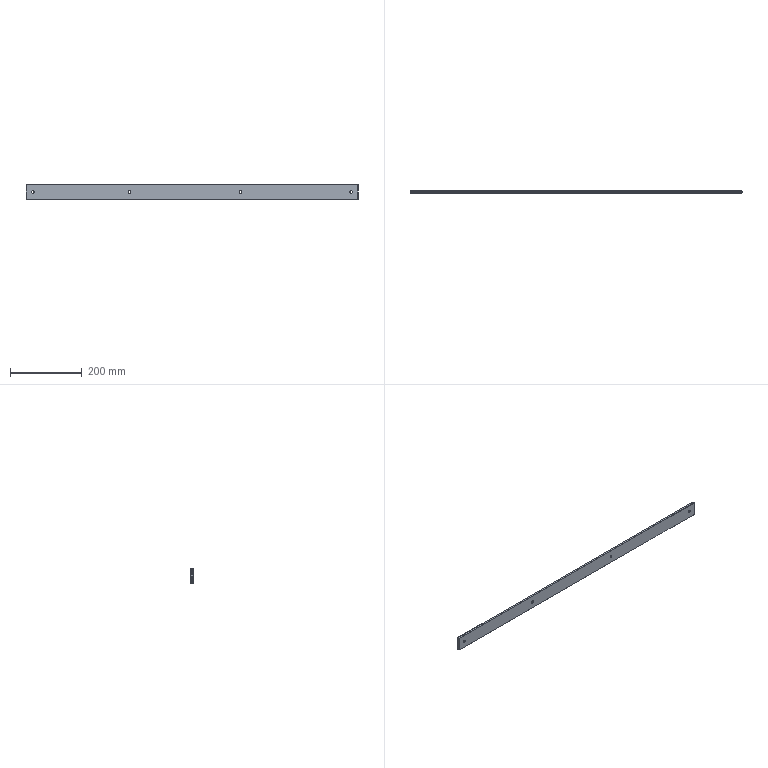Part | NX | 1 solid | 26 faces | box 928 x 6 x 40 mm | volume 221621 mm3 | plane 18 | cylinder 8 | commonest cylinder face diameters 7 x8
STEP:
#1=CARTESIAN_POINT('',(927.7,0.,-19.7));
#2=VERTEX_POINT('',#1);
#3=CARTESIAN_POINT('',(927.7,0.,19.7));
#4=VERTEX_POINT('',#3);
#5=CARTESIAN_POINT('',(927.7,0.,0.));
#6=DIRECTION('',(0.,0.,1.));
#7=VECTOR('',#6,1000.);
#8=LINE('',#5,#7);
#9=EDGE_CURVE('',#2,#4,#8,.T.);
#10=ORIENTED_EDGE('',*,*,#9,.T.);
#11=CARTESIAN_POINT('',(0.3,0.,19.7));
#12=VERTEX_POINT('',#11);
#13=CARTESIAN_POINT('',(464.,0.,19.7));
#14=DIRECTION('',(-1.,0.,0.));
#15=VECTOR('',#14,1000.);
#16=LINE('',#13,#15);
#17=EDGE_CURVE('',#4,#12,#16,.T.);
#18=ORIENTED_EDGE('',*,*,#17,.T.);
#19=CARTESIAN_POINT('',(0.3,0.,-19.7));
#20=VERTEX_POINT('',#19);
#21=CARTESIAN_POINT('',(0.3,0.,0.));
#22=DIRECTION('',(0.,0.,-1.));
#23=VECTOR('',#22,1000.);
#24=LINE('',#21,#23);
#25=EDGE_CURVE('',#12,#20,#24,.T.);
#26=ORIENTED_EDGE('',*,*,#25,.T.);
#27=CARTESIAN_POINT('',(464.,0.,-19.7));
#28=DIRECTION('',(1.,0.,0.));
#29=VECTOR('',#28,1000.);
#30=LINE('',#27,#29);
#31=EDGE_CURVE('',#20,#2,#30,.T.);
#32=ORIENTED_EDGE('',*,*,#31,.T.);
#33=EDGE_LOOP('',(#10,#18,#26,#32));
#34=FACE_BOUND('',#33,.T.);
#35=CARTESIAN_POINT('',(912.5,0.,0.));
#36=VERTEX_POINT('',#35);
#37=CARTESIAN_POINT('',(905.5,0.,0.));
#38=VERTEX_POINT('',#37);
#39=CARTESIAN_POINT('',(909.,0.,0.));
#40=DIRECTION('',(0.,-1.,0.));
#41=DIRECTION('',(-1.,0.,0.));
#42=AXIS2_PLACEMENT_3D('',#39,#40,#41);
#43=CIRCLE('',#42,3.5);
#44=EDGE_CURVE('',#36,#38,#43,.T.);
#45=ORIENTED_EDGE('',*,*,#44,.F.);
#46=CARTESIAN_POINT('',(909.,0.,0.));
#47=DIRECTION('',(0.,-1.,0.));
#48=DIRECTION('',(-1.,0.,0.));
#49=AXIS2_PLACEMENT_3D('',#46,#47,#48);
#50=CIRCLE('',#49,3.5);
#51=EDGE_CURVE('',#38,#36,#50,.T.);
#52=ORIENTED_EDGE('',*,*,#51,.F.);
#53=EDGE_LOOP('',(#45,#52));
#54=FACE_BOUND('',#53,.T.);
#55=CARTESIAN_POINT('',(595.5,0.,0.));
#56=VERTEX_POINT('',#55);
#57=CARTESIAN_POINT('',(602.5,0.,0.));
#58=VERTEX_POINT('',#57);
#59=CARTESIAN_POINT('',(599.,0.,0.));
#60=DIRECTION('',(0.,-1.,0.));
#61=DIRECTION('',(-1.,0.,0.));
#62=AXIS2_PLACEMENT_3D('',#59,#60,#61);
#63=CIRCLE('',#62,3.5);
#64=EDGE_CURVE('',#56,#58,#63,.T.);
#65=ORIENTED_EDGE('',*,*,#64,.F.);
#66=CARTESIAN_POINT('',(599.,0.,0.));
#67=DIRECTION('',(0.,-1.,0.));
#68=DIRECTION('',(-1.,0.,0.));
#69=AXIS2_PLACEMENT_3D('',#66,#67,#68);
#70=CIRCLE('',#69,3.5);
#71=EDGE_CURVE('',#58,#56,#70,.T.);
#72=ORIENTED_EDGE('',*,*,#71,.F.);
#73=EDGE_LOOP('',(#65,#72));
#74=FACE_BOUND('',#73,.T.);
#75=CARTESIAN_POINT('',(285.5,0.,0.));
#76=VERTEX_POINT('',#75);
#77=CARTESIAN_POINT('',(292.5,0.,0.));
#78=VERTEX_POINT('',#77);
#79=CARTESIAN_POINT('',(289.,0.,0.));
#80=DIRECTION('',(0.,-1.,0.));
#81=DIRECTION('',(-1.,0.,0.));
#82=AXIS2_PLACEMENT_3D('',#79,#80,#81);
#83=CIRCLE('',#82,3.5);
#84=EDGE_CURVE('',#76,#78,#83,.T.);
#85=ORIENTED_EDGE('',*,*,#84,.F.);
#86=CARTESIAN_POINT('',(289.,0.,0.));
#87=DIRECTION('',(0.,-1.,0.));
#88=DIRECTION('',(-1.,0.,0.));
#89=AXIS2_PLACEMENT_3D('',#86,#87,#88);
#90=CIRCLE('',#89,3.5);
#91=EDGE_CURVE('',#78,#76,#90,.T.);
#92=ORIENTED_EDGE('',*,*,#91,.F.);
#93=EDGE_LOOP('',(#85,#92));
#94=FACE_BOUND('',#93,.T.);
#95=CARTESIAN_POINT('',(22.5,0.,0.));
#96=VERTEX_POINT('',#95);
#97=CARTESIAN_POINT('',(15.5,0.,0.));
#98=VERTEX_POINT('',#97);
#99=CARTESIAN_POINT('',(19.,0.,0.));
#100=DIRECTION('',(0.,-1.,0.));
#101=DIRECTION('',(-1.,0.,0.));
#102=AXIS2_PLACEMENT_3D('',#99,#100,#101);
#103=CIRCLE('',#102,3.5);
#104=EDGE_CURVE('',#96,#98,#103,.T.);
#105=ORIENTED_EDGE('',*,*,#104,.F.);
#106=CARTESIAN_POINT('',(19.,0.,0.));
#107=DIRECTION('',(0.,-1.,0.));
#108=DIRECTION('',(-1.,0.,0.));
#109=AXIS2_PLACEMENT_3D('',#106,#107,#108);
#110=CIRCLE('',#109,3.5);
#111=EDGE_CURVE('',#98,#96,#110,.T.);
#112=ORIENTED_EDGE('',*,*,#111,.F.);
#113=EDGE_LOOP('',(#105,#112));
#114=FACE_BOUND('',#113,.T.);
#115=CARTESIAN_POINT('',(0.,0.,0.));
#116=DIRECTION('',(0.,1.,0.));
#117=DIRECTION('',(1.,0.,0.));
#118=AXIS2_PLACEMENT_3D('',#115,#116,#117);
#119=PLANE('',#118);
#120=ADVANCED_FACE('',(#34,#54,#74,#94,#114),#119,.F.);
#121=CARTESIAN_POINT('',(0.,5.7,19.7));
#122=VERTEX_POINT('',#121);
#123=CARTESIAN_POINT('',(0.,0.3,19.7));
#124=VERTEX_POINT('',#123);
#125=CARTESIAN_POINT('',(0.,3.,19.7));
#126=DIRECTION('',(0.,-1.,0.));
#127=VECTOR('',#126,1000.);
#128=LINE('',#125,#127);
#129=EDGE_CURVE('',#122,#124,#128,.T.);
#130=ORIENTED_EDGE('',*,*,#129,.F.);
#131=CARTESIAN_POINT('',(0.,5.7,-19.7));
#132=VERTEX_POINT('',#131);
#133=CARTESIAN_POINT('',(0.,5.7,0.));
#134=DIRECTION('',(0.,0.,-1.));
#135=VECTOR('',#134,1000.);
#136=LINE('',#133,#135);
#137=EDGE_CURVE('',#122,#132,#136,.T.);
#138=ORIENTED_EDGE('',*,*,#137,.T.);
#139=CARTESIAN_POINT('',(0.,0.3,-19.7));
#140=VERTEX_POINT('',#139);
#141=CARTESIAN_POINT('',(0.,3.,-19.7));
#142=DIRECTION('',(0.,-1.,0.));
#143=VECTOR('',#142,1000.);
#144=LINE('',#141,#143);
#145=EDGE_CURVE('',#132,#140,#144,.T.);
#146=ORIENTED_EDGE('',*,*,#145,.T.);
#147=CARTESIAN_POINT('',(0.,0.3,0.));
#148=DIRECTION('',(0.,0.,-1.));
#149=VECTOR('',#148,1000.);
#150=LINE('',#147,#149);
#151=EDGE_CURVE('',#124,#140,#150,.T.);
#152=ORIENTED_EDGE('',*,*,#151,.F.);
#153=EDGE_LOOP('',(#130,#138,#146,#152));
#154=FACE_BOUND('',#153,.T.);
#155=CARTESIAN_POINT('',(0.,0.,-20.));
#156=DIRECTION('',(-1.,0.,0.));
#157=DIRECTION('',(0.,0.,1.));
#158=AXIS2_PLACEMENT_3D('',#155,#156,#157);
#159=PLANE('',#158);
#160=ADVANCED_FACE('',(#154),#159,.T.);
#161=CARTESIAN_POINT('',(927.7,5.7,-20.));
#162=VERTEX_POINT('',#161);
#163=CARTESIAN_POINT('',(927.7,0.3,-20.));
#164=VERTEX_POINT('',#163);
#165=CARTESIAN_POINT('',(927.7,3.,-20.));
#166=DIRECTION('',(0.,-1.,0.));
#167=VECTOR('',#166,1000.);
#168=LINE('',#165,#167);
#169=EDGE_CURVE('',#162,#164,#168,.T.);
#170=ORIENTED_EDGE('',*,*,#169,.T.);
#171=CARTESIAN_POINT('',(0.3,0.3,-20.));
#172=VERTEX_POINT('',#171);
#173=CARTESIAN_POINT('',(464.,0.3,-20.));
#174=DIRECTION('',(1.,0.,0.));
#175=VECTOR('',#174,1000.);
#176=LINE('',#173,#175);
#177=EDGE_CURVE('',#172,#164,#176,.T.);
#178=ORIENTED_EDGE('',*,*,#177,.F.);
#179=CARTESIAN_POINT('',(0.3,5.7,-20.));
#180=VERTEX_POINT('',#179);
#181=CARTESIAN_POINT('',(0.3,3.,-20.));
#182=DIRECTION('',(0.,-1.,0.));
#183=VECTOR('',#182,1000.);
#184=LINE('',#181,#183);
#185=EDGE_CURVE('',#180,#172,#184,.T.);
#186=ORIENTED_EDGE('',*,*,#185,.F.);
#187=CARTESIAN_POINT('',(464.,5.7,-20.));
#188=DIRECTION('',(1.,0.,0.));
#189=VECTOR('',#188,1000.);
#190=LINE('',#187,#189);
#191=EDGE_CURVE('',#180,#162,#190,.T.);
#192=ORIENTED_EDGE('',*,*,#191,.T.);
#193=EDGE_LOOP('',(#170,#178,#186,#192));
#194=FACE_BOUND('',#193,.T.);
#195=CARTESIAN_POINT('',(928.,0.,-20.));
#196=DIRECTION('',(0.,0.,-1.));
#197=DIRECTION('',(0.,-1.,0.));
#198=AXIS2_PLACEMENT_3D('',#195,#196,#197);
#199=PLANE('',#198);
#200=ADVANCED_FACE('',(#194),#199,.T.);
#201=CARTESIAN_POINT('',(928.,5.7,-19.7));
#202=VERTEX_POINT('',#201);
#203=CARTESIAN_POINT('',(928.,5.7,19.7));
#204=VERTEX_POINT('',#203);
#205=CARTESIAN_POINT('',(928.,5.7,0.));
#206=DIRECTION('',(0.,0.,1.));
#207=VECTOR('',#206,1000.);
#208=LINE('',#205,#207);
#209=EDGE_CURVE('',#202,#204,#208,.T.);
#210=ORIENTED_EDGE('',*,*,#209,.T.);
#211=CARTESIAN_POINT('',(928.,0.3,19.7));
#212=VERTEX_POINT('',#211);
#213=CARTESIAN_POINT('',(928.,3.,19.7));
#214=DIRECTION('',(0.,-1.,0.));
#215=VECTOR('',#214,1000.);
#216=LINE('',#213,#215);
#217=EDGE_CURVE('',#204,#212,#216,.T.);
#218=ORIENTED_EDGE('',*,*,#217,.T.);
#219=CARTESIAN_POINT('',(928.,0.3,-19.7));
#220=VERTEX_POINT('',#219);
#221=CARTESIAN_POINT('',(928.,0.3,0.));
#222=DIRECTION('',(0.,0.,1.));
#223=VECTOR('',#222,1000.);
#224=LINE('',#221,#223);
#225=EDGE_CURVE('',#220,#212,#224,.T.);
#226=ORIENTED_EDGE('',*,*,#225,.F.);
#227=CARTESIAN_POINT('',(928.,3.,-19.7));
#228=DIRECTION('',(0.,-1.,0.));
#229=VECTOR('',#228,1000.);
#230=LINE('',#227,#229);
#231=EDGE_CURVE('',#202,#220,#230,.T.);
#232=ORIENTED_EDGE('',*,*,#231,.F.);
#233=EDGE_LOOP('',(#210,#218,#226,#232));
#234=FACE_BOUND('',#233,.T.);
#235=CARTESIAN_POINT('',(928.,0.,20.));
#236=DIRECTION('',(1.,0.,0.));
#237=DIRECTION('',(0.,1.,0.));
#238=AXIS2_PLACEMENT_3D('',#235,#236,#237);
#239=PLANE('',#238);
#240=ADVANCED_FACE('',(#234),#239,.T.);
#241=CARTESIAN_POINT('',(927.7,5.7,20.));
#242=VERTEX_POINT('',#241);
#243=CARTESIAN_POINT('',(0.3,5.7,20.));
#244=VERTEX_POINT('',#243);
#245=CARTESIAN_POINT('',(464.,5.7,20.));
#246=DIRECTION('',(-1.,0.,0.));
#247=VECTOR('',#246,1000.);
#248=LINE('',#245,#247);
#249=EDGE_CURVE('',#242,#244,#248,.T.);
#250=ORIENTED_EDGE('',*,*,#249,.T.);
#251=CARTESIAN_POINT('',(0.3,0.3,20.));
#252=VERTEX_POINT('',#251);
#253=CARTESIAN_POINT('',(0.3,3.,20.));
#254=DIRECTION('',(0.,-1.,0.));
#255=VECTOR('',#254,1000.);
#256=LINE('',#253,#255);
#257=EDGE_CURVE('',#244,#252,#256,.T.);
#258=ORIENTED_EDGE('',*,*,#257,.T.);
#259=CARTESIAN_POINT('',(927.7,0.3,20.));
#260=VERTEX_POINT('',#259);
#261=CARTESIAN_POINT('',(464.,0.3,20.));
#262=DIRECTION('',(-1.,0.,0.));
#263=VECTOR('',#262,1000.);
#264=LINE('',#261,#263);
#265=EDGE_CURVE('',#260,#252,#264,.T.);
#266=ORIENTED_EDGE('',*,*,#265,.F.);
#267=CARTESIAN_POINT('',(927.7,3.,20.));
#268=DIRECTION('',(0.,-1.,0.));
#269=VECTOR('',#268,1000.);
#270=LINE('',#267,#269);
#271=EDGE_CURVE('',#242,#260,#270,.T.);
#272=ORIENTED_EDGE('',*,*,#271,.F.);
#273=EDGE_LOOP('',(#250,#258,#266,#272));
#274=FACE_BOUND('',#273,.T.);
#275=CARTESIAN_POINT('',(0.,0.,20.));
#276=DIRECTION('',(0.,0.,1.));
#277=DIRECTION('',(1.,0.,0.));
#278=AXIS2_PLACEMENT_3D('',#275,#276,#277);
#279=PLANE('',#278);
#280=ADVANCED_FACE('',(#274),#279,.T.);
#281=CARTESIAN_POINT('',(0.3,6.,19.7));
#282=VERTEX_POINT('',#281);
#283=CARTESIAN_POINT('',(0.3,6.,-19.7));
#284=VERTEX_POINT('',#283);
#285=CARTESIAN_POINT('',(0.3,6.,0.));
#286=DIRECTION('',(0.,0.,-1.));
#287=VECTOR('',#286,1000.);
#288=LINE('',#285,#287);
#289=EDGE_CURVE('',#282,#284,#288,.T.);
#290=ORIENTED_EDGE('',*,*,#289,.F.);
#291=CARTESIAN_POINT('',(927.7,6.,19.7));
#292=VERTEX_POINT('',#291);
#293=CARTESIAN_POINT('',(464.,6.,19.7));
#294=DIRECTION('',(-1.,0.,0.));
#295=VECTOR('',#294,1000.);
#296=LINE('',#293,#295);
#297=EDGE_CURVE('',#292,#282,#296,.T.);
#298=ORIENTED_EDGE('',*,*,#297,.F.);
#299=CARTESIAN_POINT('',(927.7,6.,-19.7));
#300=VERTEX_POINT('',#299);
#301=CARTESIAN_POINT('',(927.7,6.,0.));
#302=DIRECTION('',(0.,0.,1.));
#303=VECTOR('',#302,1000.);
#304=LINE('',#301,#303);
#305=EDGE_CURVE('',#300,#292,#304,.T.);
#306=ORIENTED_EDGE('',*,*,#305,.F.);
#307=CARTESIAN_POINT('',(464.,6.,-19.7));
#308=DIRECTION('',(1.,0.,0.));
#309=VECTOR('',#308,1000.);
#310=LINE('',#307,#309);
#311=EDGE_CURVE('',#284,#300,#310,.T.);
#312=ORIENTED_EDGE('',*,*,#311,.F.);
#313=EDGE_LOOP('',(#290,#298,#306,#312));
#314=FACE_BOUND('',#313,.T.);
#315=CARTESIAN_POINT('',(905.5,6.,0.));
#316=VERTEX_POINT('',#315);
#317=CARTESIAN_POINT('',(912.5,6.,0.));
#318=VERTEX_POINT('',#317);
#319=CARTESIAN_POINT('',(909.,6.,0.));
#320=DIRECTION('',(0.,1.,0.));
#321=DIRECTION('',(1.,0.,0.));
#322=AXIS2_PLACEMENT_3D('',#319,#320,#321);
#323=CIRCLE('',#322,3.5);
#324=EDGE_CURVE('',#316,#318,#323,.T.);
#325=ORIENTED_EDGE('',*,*,#324,.F.);
#326=CARTESIAN_POINT('',(909.,6.,0.));
#327=DIRECTION('',(0.,1.,0.));
#328=DIRECTION('',(1.,0.,0.));
#329=AXIS2_PLACEMENT_3D('',#326,#327,#328);
#330=CIRCLE('',#329,3.5);
#331=EDGE_CURVE('',#318,#316,#330,.T.);
#332=ORIENTED_EDGE('',*,*,#331,.F.);
#333=EDGE_LOOP('',(#325,#332));
#334=FACE_BOUND('',#333,.T.);
#335=CARTESIAN_POINT('',(595.5,6.,0.));
#336=VERTEX_POINT('',#335);
#337=CARTESIAN_POINT('',(602.5,6.,0.));
#338=VERTEX_POINT('',#337);
#339=CARTESIAN_POINT('',(599.,6.,0.));
#340=DIRECTION('',(0.,1.,0.));
#341=DIRECTION('',(1.,0.,0.));
#342=AXIS2_PLACEMENT_3D('',#339,#340,#341);
#343=CIRCLE('',#342,3.5);
#344=EDGE_CURVE('',#336,#338,#343,.T.);
#345=ORIENTED_EDGE('',*,*,#344,.F.);
#346=CARTESIAN_POINT('',(599.,6.,0.));
#347=DIRECTION('',(0.,1.,0.));
#348=DIRECTION('',(1.,0.,0.));
#349=AXIS2_PLACEMENT_3D('',#346,#347,#348);
#350=CIRCLE('',#349,3.5);
#351=EDGE_CURVE('',#338,#336,#350,.T.);
#352=ORIENTED_EDGE('',*,*,#351,.F.);
#353=EDGE_LOOP('',(#345,#352));
#354=FACE_BOUND('',#353,.T.);
#355=CARTESIAN_POINT('',(292.5,6.,0.));
#356=VERTEX_POINT('',#355);
#357=CARTESIAN_POINT('',(285.5,6.,0.));
#358=VERTEX_POINT('',#357);
#359=CARTESIAN_POINT('',(289.,6.,0.));
#360=DIRECTION('',(0.,1.,0.));
#361=DIRECTION('',(1.,0.,0.));
#362=AXIS2_PLACEMENT_3D('',#359,#360,#361);
#363=CIRCLE('',#362,3.5);
#364=EDGE_CURVE('',#356,#358,#363,.T.);
#365=ORIENTED_EDGE('',*,*,#364,.F.);
#366=CARTESIAN_POINT('',(289.,6.,0.));
#367=DIRECTION('',(0.,1.,0.));
#368=DIRECTION('',(1.,0.,0.));
#369=AXIS2_PLACEMENT_3D('',#366,#367,#368);
#370=CIRCLE('',#369,3.5);
#371=EDGE_CURVE('',#358,#356,#370,.T.);
#372=ORIENTED_EDGE('',*,*,#371,.F.);
#373=EDGE_LOOP('',(#365,#372));
#374=FACE_BOUND('',#373,.T.);
#375=CARTESIAN_POINT('',(22.5,6.,0.));
#376=VERTEX_POINT('',#375);
#377=CARTESIAN_POINT('',(15.5,6.,0.));
#378=VERTEX_POINT('',#377);
#379=CARTESIAN_POINT('',(19.,6.,0.));
#380=DIRECTION('',(0.,1.,0.));
#381=DIRECTION('',(1.,0.,0.));
#382=AXIS2_PLACEMENT_3D('',#379,#380,#381);
#383=CIRCLE('',#382,3.5);
#384=EDGE_CURVE('',#376,#378,#383,.T.);
#385=ORIENTED_EDGE('',*,*,#384,.F.);
#386=CARTESIAN_POINT('',(19.,6.,0.));
#387=DIRECTION('',(0.,1.,0.));
#388=DIRECTION('',(1.,0.,0.));
#389=AXIS2_PLACEMENT_3D('',#386,#387,#388);
#390=CIRCLE('',#389,3.5);
#391=EDGE_CURVE('',#378,#376,#390,.T.);
#392=ORIENTED_EDGE('',*,*,#391,.F.);
#393=EDGE_LOOP('',(#385,#392));
#394=FACE_BOUND('',#393,.T.);
#395=CARTESIAN_POINT('',(0.,6.,0.));
#396=DIRECTION('',(0.,1.,0.));
#397=DIRECTION('',(1.,0.,0.));
#398=AXIS2_PLACEMENT_3D('',#395,#396,#397);
#399=PLANE('',#398);
#400=ADVANCED_FACE('',(#314,#334,#354,#374,#394),#399,.T.);
#401=ORIENTED_EDGE('',*,*,#384,.T.);
#402=CARTESIAN_POINT('',(15.5,6.,0.));
#403=DIRECTION('',(0.,-1.,0.));
#404=VECTOR('',#403,1000.);
#405=LINE('',#402,#404);
#406=EDGE_CURVE('',#98,#378,#405,.F.);
#407=ORIENTED_EDGE('',*,*,#406,.F.);
#408=ORIENTED_EDGE('',*,*,#111,.T.);
#409=CARTESIAN_POINT('',(22.5,6.,0.));
#410=DIRECTION('',(0.,-1.,0.));
#411=VECTOR('',#410,1000.);
#412=LINE('',#409,#411);
#413=EDGE_CURVE('',#96,#376,#412,.F.);
#414=ORIENTED_EDGE('',*,*,#413,.T.);
#415=EDGE_LOOP('',(#401,#407,#408,#414));
#416=FACE_BOUND('',#415,.T.);
#417=CARTESIAN_POINT('',(19.,6.,0.));
#418=DIRECTION('',(0.,-1.,0.));
#419=DIRECTION('',(1.,0.,0.));
#420=AXIS2_PLACEMENT_3D('',#417,#418,#419);
#421=CYLINDRICAL_SURFACE('',#420,3.5);
#422=ADVANCED_FACE('',(#416),#421,.F.);
#423=ORIENTED_EDGE('',*,*,#344,.T.);
#424=CARTESIAN_POINT('',(602.5,0.,0.));
#425=DIRECTION('',(0.,1.,0.));
#426=VECTOR('',#425,1000.);
#427=LINE('',#424,#426);
#428=EDGE_CURVE('',#58,#338,#427,.T.);
#429=ORIENTED_EDGE('',*,*,#428,.F.);
#430=ORIENTED_EDGE('',*,*,#71,.T.);
#431=CARTESIAN_POINT('',(595.5,0.,0.));
#432=DIRECTION('',(0.,1.,0.));
#433=VECTOR('',#432,1000.);
#434=LINE('',#431,#433);
#435=EDGE_CURVE('',#56,#336,#434,.T.);
#436=ORIENTED_EDGE('',*,*,#435,.T.);
#437=EDGE_LOOP('',(#423,#429,#430,#436));
#438=FACE_BOUND('',#437,.T.);
#439=CARTESIAN_POINT('',(599.,0.,0.));
#440=DIRECTION('',(0.,1.,0.));
#441=DIRECTION('',(-1.,0.,0.));
#442=AXIS2_PLACEMENT_3D('',#439,#440,#441);
#443=CYLINDRICAL_SURFACE('',#442,3.5);
#444=ADVANCED_FACE('',(#438),#443,.F.);
#445=ORIENTED_EDGE('',*,*,#44,.T.);
#446=CARTESIAN_POINT('',(905.5,0.,0.));
#447=DIRECTION('',(0.,1.,0.));
#448=VECTOR('',#447,1000.);
#449=LINE('',#446,#448);
#450=EDGE_CURVE('',#316,#38,#449,.F.);
#451=ORIENTED_EDGE('',*,*,#450,.F.);
#452=ORIENTED_EDGE('',*,*,#324,.T.);
#453=CARTESIAN_POINT('',(912.5,0.,0.));
#454=DIRECTION('',(0.,1.,0.));
#455=VECTOR('',#454,1000.);
#456=LINE('',#453,#455);
#457=EDGE_CURVE('',#318,#36,#456,.F.);
#458=ORIENTED_EDGE('',*,*,#457,.T.);
#459=EDGE_LOOP('',(#445,#451,#452,#458));
#460=FACE_BOUND('',#459,.T.);
#461=CARTESIAN_POINT('',(909.,0.,0.));
#462=DIRECTION('',(0.,1.,0.));
#463=DIRECTION('',(-1.,0.,0.));
#464=AXIS2_PLACEMENT_3D('',#461,#462,#463);
#465=CYLINDRICAL_SURFACE('',#464,3.5);
#466=ADVANCED_FACE('',(#460),#465,.F.);
#467=ORIENTED_EDGE('',*,*,#84,.T.);
#468=CARTESIAN_POINT('',(292.5,0.,0.));
#469=DIRECTION('',(0.,1.,0.));
#470=VECTOR('',#469,1000.);
#471=LINE('',#468,#470);
#472=EDGE_CURVE('',#356,#78,#471,.F.);
#473=ORIENTED_EDGE('',*,*,#472,.F.);
#474=ORIENTED_EDGE('',*,*,#364,.T.);
#475=CARTESIAN_POINT('',(285.5,0.,0.));
#476=DIRECTION('',(0.,1.,0.));
#477=VECTOR('',#476,1000.);
#478=LINE('',#475,#477);
#479=EDGE_CURVE('',#358,#76,#478,.F.);
#480=ORIENTED_EDGE('',*,*,#479,.T.);
#481=EDGE_LOOP('',(#467,#473,#474,#480));
#482=FACE_BOUND('',#481,.T.);
#483=CARTESIAN_POINT('',(289.,0.,0.));
#484=DIRECTION('',(0.,1.,0.));
#485=DIRECTION('',(-1.,0.,0.));
#486=AXIS2_PLACEMENT_3D('',#483,#484,#485);
#487=CYLINDRICAL_SURFACE('',#486,3.5);
#488=ADVANCED_FACE('',(#482),#487,.F.);
#489=ORIENTED_EDGE('',*,*,#191,.F.);
#490=CARTESIAN_POINT('',(0.15,5.85,-19.85));
#491=VERTEX_POINT('',#490);
#492=CARTESIAN_POINT('',(-19.7,25.7,0.));
#493=DIRECTION('',(-0.5774,0.5774,0.5774));
#494=VECTOR('',#493,1000.);
#495=LINE('',#492,#494);
#496=EDGE_CURVE('',#180,#491,#495,.T.);
#497=ORIENTED_EDGE('',*,*,#496,.T.);
#498=CARTESIAN_POINT('',(20.,25.7,0.));
#499=DIRECTION('',(0.5774,0.5774,0.5774));
#500=VECTOR('',#499,1000.);
#501=LINE('',#498,#500);
#502=EDGE_CURVE('',#491,#284,#501,.T.);
#503=ORIENTED_EDGE('',*,*,#502,.T.);
#504=ORIENTED_EDGE('',*,*,#311,.T.);
#505=CARTESIAN_POINT('',(927.85,5.85,-19.85));
#506=VERTEX_POINT('',#505);
#507=CARTESIAN_POINT('',(908.,25.7,0.));
#508=DIRECTION('',(0.5774,-0.5774,-0.5774));
#509=VECTOR('',#508,1000.);
#510=LINE('',#507,#509);
#511=EDGE_CURVE('',#300,#506,#510,.T.);
#512=ORIENTED_EDGE('',*,*,#511,.T.);
#513=CARTESIAN_POINT('',(947.7,25.7,0.));
#514=DIRECTION('',(-0.5774,-0.5774,-0.5774));
#515=VECTOR('',#514,1000.);
#516=LINE('',#513,#515);
#517=EDGE_CURVE('',#506,#162,#516,.T.);
#518=ORIENTED_EDGE('',*,*,#517,.T.);
#519=EDGE_LOOP('',(#489,#497,#503,#504,#512,#518));
#520=FACE_BOUND('',#519,.T.);
#521=CARTESIAN_POINT('',(464.,5.85,-19.85));
#522=DIRECTION('',(0.,0.7071,-0.7071));
#523=DIRECTION('',(-1.,0.,0.));
#524=AXIS2_PLACEMENT_3D('',#521,#522,#523);
#525=PLANE('',#524);
#526=ADVANCED_FACE('',(#520),#525,.T.);
#527=ORIENTED_EDGE('',*,*,#145,.F.);
#528=CARTESIAN_POINT('',(-19.7,-14.,0.));
#529=DIRECTION('',(0.5774,0.5774,-0.5774));
#530=VECTOR('',#529,1000.);
#531=LINE('',#528,#530);
#532=EDGE_CURVE('',#132,#491,#531,.T.);
#533=ORIENTED_EDGE('',*,*,#532,.T.);
#534=ORIENTED_EDGE('',*,*,#496,.F.);
#535=ORIENTED_EDGE('',*,*,#185,.T.);
#536=CARTESIAN_POINT('',(0.15,0.15,-19.85));
#537=VERTEX_POINT('',#536);
#538=CARTESIAN_POINT('',(-19.7,-19.7,0.));
#539=DIRECTION('',(-0.5774,-0.5774,0.5774));
#540=VECTOR('',#539,1000.);
#541=LINE('',#538,#540);
#542=EDGE_CURVE('',#172,#537,#541,.T.);
#543=ORIENTED_EDGE('',*,*,#542,.T.);
#544=CARTESIAN_POINT('',(-19.7,20.,0.));
#545=DIRECTION('',(-0.5774,0.5774,0.5774));
#546=VECTOR('',#545,1000.);
#547=LINE('',#544,#546);
#548=EDGE_CURVE('',#537,#140,#547,.T.);
#549=ORIENTED_EDGE('',*,*,#548,.T.);
#550=EDGE_LOOP('',(#527,#533,#534,#535,#543,#549));
#551=FACE_BOUND('',#550,.T.);
#552=CARTESIAN_POINT('',(0.15,3.,-19.85));
#553=DIRECTION('',(-0.7071,0.,-0.7071));
#554=DIRECTION('',(-0.7071,0.,0.7071));
#555=AXIS2_PLACEMENT_3D('',#552,#553,#554);
#556=PLANE('',#555);
#557=ADVANCED_FACE('',(#551),#556,.T.);
#558=ORIENTED_EDGE('',*,*,#25,.F.);
#559=CARTESIAN_POINT('',(0.15,0.15,19.85));
#560=VERTEX_POINT('',#559);
#561=CARTESIAN_POINT('',(20.,-19.7,0.));
#562=DIRECTION('',(-0.5774,0.5774,0.5774));
#563=VECTOR('',#562,1000.);
#564=LINE('',#561,#563);
#565=EDGE_CURVE('',#12,#560,#564,.T.);
#566=ORIENTED_EDGE('',*,*,#565,.T.);
#567=CARTESIAN_POINT('',(0.3,0.,20.));
#568=DIRECTION('',(0.5774,-0.5774,0.5774));
#569=VECTOR('',#568,1000.);
#570=LINE('',#567,#569);
#571=EDGE_CURVE('',#124,#560,#570,.T.);
#572=ORIENTED_EDGE('',*,*,#571,.F.);
#573=ORIENTED_EDGE('',*,*,#151,.T.);
#574=ORIENTED_EDGE('',*,*,#548,.F.);
#575=CARTESIAN_POINT('',(20.,-19.7,0.));
#576=DIRECTION('',(0.5774,-0.5774,0.5774));
#577=VECTOR('',#576,1000.);
#578=LINE('',#575,#577);
#579=EDGE_CURVE('',#537,#20,#578,.T.);
#580=ORIENTED_EDGE('',*,*,#579,.T.);
#581=EDGE_LOOP('',(#558,#566,#572,#573,#574,#580));
#582=FACE_BOUND('',#581,.T.);
#583=CARTESIAN_POINT('',(0.15,0.15,0.));
#584=DIRECTION('',(-0.7071,-0.7071,0.));
#585=DIRECTION('',(-0.7071,0.7071,0.));
#586=AXIS2_PLACEMENT_3D('',#583,#584,#585);
#587=PLANE('',#586);
#588=ADVANCED_FACE('',(#582),#587,.T.);
#589=ORIENTED_EDGE('',*,*,#137,.F.);
#590=CARTESIAN_POINT('',(0.15,5.85,19.85));
#591=VERTEX_POINT('',#590);
#592=CARTESIAN_POINT('',(0.,5.7,19.7));
#593=DIRECTION('',(-0.5774,-0.5774,-0.5774));
#594=VECTOR('',#593,1000.);
#595=LINE('',#592,#594);
#596=EDGE_CURVE('',#591,#122,#595,.T.);
#597=ORIENTED_EDGE('',*,*,#596,.F.);
#598=CARTESIAN_POINT('',(20.,25.7,0.));
#599=DIRECTION('',(0.5774,0.5774,-0.5774));
#600=VECTOR('',#599,1000.);
#601=LINE('',#598,#600);
#602=EDGE_CURVE('',#591,#282,#601,.T.);
#603=ORIENTED_EDGE('',*,*,#602,.T.);
#604=ORIENTED_EDGE('',*,*,#289,.T.);
#605=ORIENTED_EDGE('',*,*,#502,.F.);
#606=ORIENTED_EDGE('',*,*,#532,.F.);
#607=EDGE_LOOP('',(#589,#597,#603,#604,#605,#606));
#608=FACE_BOUND('',#607,.T.);
#609=CARTESIAN_POINT('',(0.15,5.85,0.));
#610=DIRECTION('',(-0.7071,0.7071,0.));
#611=DIRECTION('',(0.,0.,1.));
#612=AXIS2_PLACEMENT_3D('',#609,#610,#611);
#613=PLANE('',#612);
#614=ADVANCED_FACE('',(#608),#613,.T.);
#615=ORIENTED_EDGE('',*,*,#31,.F.);
#616=ORIENTED_EDGE('',*,*,#579,.F.);
#617=ORIENTED_EDGE('',*,*,#542,.F.);
#618=ORIENTED_EDGE('',*,*,#177,.T.);
#619=CARTESIAN_POINT('',(927.85,0.15,-19.85));
#620=VERTEX_POINT('',#619);
#621=CARTESIAN_POINT('',(947.7,-19.7,0.));
#622=DIRECTION('',(0.5774,-0.5774,0.5774));
#623=VECTOR('',#622,1000.);
#624=LINE('',#621,#623);
#625=EDGE_CURVE('',#164,#620,#624,.T.);
#626=ORIENTED_EDGE('',*,*,#625,.T.);
#627=CARTESIAN_POINT('',(908.,-19.7,0.));
#628=DIRECTION('',(-0.5774,-0.5774,0.5774));
#629=VECTOR('',#628,1000.);
#630=LINE('',#627,#629);
#631=EDGE_CURVE('',#620,#2,#630,.T.);
#632=ORIENTED_EDGE('',*,*,#631,.T.);
#633=EDGE_LOOP('',(#615,#616,#617,#618,#626,#632));
#634=FACE_BOUND('',#633,.T.);
#635=CARTESIAN_POINT('',(464.,0.15,-19.85));
#636=DIRECTION('',(0.,-0.7071,-0.7071));
#637=DIRECTION('',(0.,0.7071,-0.7071));
#638=AXIS2_PLACEMENT_3D('',#635,#636,#637);
#639=PLANE('',#638);
#640=ADVANCED_FACE('',(#634),#639,.T.);
#641=ORIENTED_EDGE('',*,*,#129,.T.);
#642=ORIENTED_EDGE('',*,*,#571,.T.);
#643=CARTESIAN_POINT('',(0.,0.,19.7));
#644=DIRECTION('',(-0.5774,-0.5774,-0.5774));
#645=VECTOR('',#644,1000.);
#646=LINE('',#643,#645);
#647=EDGE_CURVE('',#252,#560,#646,.T.);
#648=ORIENTED_EDGE('',*,*,#647,.F.);
#649=ORIENTED_EDGE('',*,*,#257,.F.);
#650=CARTESIAN_POINT('',(0.,6.,19.7));
#651=DIRECTION('',(0.5774,-0.5774,0.5774));
#652=VECTOR('',#651,1000.);
#653=LINE('',#650,#652);
#654=EDGE_CURVE('',#591,#244,#653,.T.);
#655=ORIENTED_EDGE('',*,*,#654,.F.);
#656=ORIENTED_EDGE('',*,*,#596,.T.);
#657=EDGE_LOOP('',(#641,#642,#648,#649,#655,#656));
#658=FACE_BOUND('',#657,.T.);
#659=CARTESIAN_POINT('',(0.15,3.,19.85));
#660=DIRECTION('',(0.7071,0.,-0.7071));
#661=DIRECTION('',(0.,-1.,0.));
#662=AXIS2_PLACEMENT_3D('',#659,#660,#661);
#663=PLANE('',#662);
#664=ADVANCED_FACE('',(#658),#663,.F.);
#665=ORIENTED_EDGE('',*,*,#249,.F.);
#666=CARTESIAN_POINT('',(927.85,5.85,19.85));
#667=VERTEX_POINT('',#666);
#668=CARTESIAN_POINT('',(947.7,25.7,0.));
#669=DIRECTION('',(0.5774,0.5774,-0.5774));
#670=VECTOR('',#669,1000.);
#671=LINE('',#668,#670);
#672=EDGE_CURVE('',#242,#667,#671,.T.);
#673=ORIENTED_EDGE('',*,*,#672,.T.);
#674=CARTESIAN_POINT('',(908.,25.7,0.));
#675=DIRECTION('',(-0.5774,0.5774,-0.5774));
#676=VECTOR('',#675,1000.);
#677=LINE('',#674,#676);
#678=EDGE_CURVE('',#667,#292,#677,.T.);
#679=ORIENTED_EDGE('',*,*,#678,.T.);
#680=ORIENTED_EDGE('',*,*,#297,.T.);
#681=ORIENTED_EDGE('',*,*,#602,.F.);
#682=ORIENTED_EDGE('',*,*,#654,.T.);
#683=EDGE_LOOP('',(#665,#673,#679,#680,#681,#682));
#684=FACE_BOUND('',#683,.T.);
#685=CARTESIAN_POINT('',(464.,5.85,19.85));
#686=DIRECTION('',(0.,0.7071,0.7071));
#687=DIRECTION('',(1.,0.,0.));
#688=AXIS2_PLACEMENT_3D('',#685,#686,#687);
#689=PLANE('',#688);
#690=ADVANCED_FACE('',(#684),#689,.T.);
#691=ORIENTED_EDGE('',*,*,#17,.F.);
#692=CARTESIAN_POINT('',(927.85,0.15,19.85));
#693=VERTEX_POINT('',#692);
#694=CARTESIAN_POINT('',(908.,-19.7,0.));
#695=DIRECTION('',(0.5774,0.5774,0.5774));
#696=VECTOR('',#695,1000.);
#697=LINE('',#694,#696);
#698=EDGE_CURVE('',#4,#693,#697,.T.);
#699=ORIENTED_EDGE('',*,*,#698,.T.);
#700=CARTESIAN_POINT('',(947.7,-19.7,0.));
#701=DIRECTION('',(-0.5774,0.5774,0.5774));
#702=VECTOR('',#701,1000.);
#703=LINE('',#700,#702);
#704=EDGE_CURVE('',#693,#260,#703,.T.);
#705=ORIENTED_EDGE('',*,*,#704,.T.);
#706=ORIENTED_EDGE('',*,*,#265,.T.);
#707=ORIENTED_EDGE('',*,*,#647,.T.);
#708=ORIENTED_EDGE('',*,*,#565,.F.);
#709=EDGE_LOOP('',(#691,#699,#705,#706,#707,#708));
#710=FACE_BOUND('',#709,.T.);
#711=CARTESIAN_POINT('',(464.,0.15,19.85));
#712=DIRECTION('',(0.,-0.7071,0.7071));
#713=DIRECTION('',(-1.,0.,0.));
#714=AXIS2_PLACEMENT_3D('',#711,#712,#713);
#715=PLANE('',#714);
#716=ADVANCED_FACE('',(#710),#715,.T.);
#717=ORIENTED_EDGE('',*,*,#217,.F.);
#718=CARTESIAN_POINT('',(947.7,-14.,0.));
#719=DIRECTION('',(-0.5774,0.5774,0.5774));
#720=VECTOR('',#719,1000.);
#721=LINE('',#718,#720);
#722=EDGE_CURVE('',#204,#667,#721,.T.);
#723=ORIENTED_EDGE('',*,*,#722,.T.);
#724=ORIENTED_EDGE('',*,*,#672,.F.);
#725=ORIENTED_EDGE('',*,*,#271,.T.);
#726=ORIENTED_EDGE('',*,*,#704,.F.);
#727=CARTESIAN_POINT('',(947.7,20.,0.));
#728=DIRECTION('',(0.5774,0.5774,-0.5774));
#729=VECTOR('',#728,1000.);
#730=LINE('',#727,#729);
#731=EDGE_CURVE('',#693,#212,#730,.T.);
#732=ORIENTED_EDGE('',*,*,#731,.T.);
#733=EDGE_LOOP('',(#717,#723,#724,#725,#726,#732));
#734=FACE_BOUND('',#733,.T.);
#735=CARTESIAN_POINT('',(927.85,3.,19.85));
#736=DIRECTION('',(0.7071,0.,0.7071));
#737=DIRECTION('',(0.,-1.,0.));
#738=AXIS2_PLACEMENT_3D('',#735,#736,#737);
#739=PLANE('',#738);
#740=ADVANCED_FACE('',(#734),#739,.T.);
#741=ORIENTED_EDGE('',*,*,#9,.F.);
#742=ORIENTED_EDGE('',*,*,#631,.F.);
#743=CARTESIAN_POINT('',(927.7,0.,-20.));
#744=DIRECTION('',(0.5774,0.5774,0.5774));
#745=VECTOR('',#744,1000.);
#746=LINE('',#743,#745);
#747=EDGE_CURVE('',#620,#220,#746,.T.);
#748=ORIENTED_EDGE('',*,*,#747,.T.);
#749=ORIENTED_EDGE('',*,*,#225,.T.);
#750=ORIENTED_EDGE('',*,*,#731,.F.);
#751=ORIENTED_EDGE('',*,*,#698,.F.);
#752=EDGE_LOOP('',(#741,#742,#748,#749,#750,#751));
#753=FACE_BOUND('',#752,.T.);
#754=CARTESIAN_POINT('',(927.85,0.15,0.));
#755=DIRECTION('',(0.7071,-0.7071,0.));
#756=DIRECTION('',(0.,0.,-1.));
#757=AXIS2_PLACEMENT_3D('',#754,#755,#756);
#758=PLANE('',#757);
#759=ADVANCED_FACE('',(#753),#758,.T.);
#760=ORIENTED_EDGE('',*,*,#209,.F.);
#761=CARTESIAN_POINT('',(933.7,0.,-14.));
#762=DIRECTION('',(-0.5774,0.5774,-0.5774));
#763=VECTOR('',#762,1000.);
#764=LINE('',#761,#763);
#765=EDGE_CURVE('',#202,#506,#764,.T.);
#766=ORIENTED_EDGE('',*,*,#765,.T.);
#767=ORIENTED_EDGE('',*,*,#511,.F.);
#768=ORIENTED_EDGE('',*,*,#305,.T.);
#769=ORIENTED_EDGE('',*,*,#678,.F.);
#770=ORIENTED_EDGE('',*,*,#722,.F.);
#771=EDGE_LOOP('',(#760,#766,#767,#768,#769,#770));
#772=FACE_BOUND('',#771,.T.);
#773=CARTESIAN_POINT('',(927.85,5.85,0.));
#774=DIRECTION('',(0.7071,0.7071,0.));
#775=DIRECTION('',(0.,0.,-1.));
#776=AXIS2_PLACEMENT_3D('',#773,#774,#775);
#777=PLANE('',#776);
#778=ADVANCED_FACE('',(#772),#777,.T.);
#779=ORIENTED_EDGE('',*,*,#169,.F.);
#780=ORIENTED_EDGE('',*,*,#517,.F.);
#781=ORIENTED_EDGE('',*,*,#765,.F.);
#782=ORIENTED_EDGE('',*,*,#231,.T.);
#783=ORIENTED_EDGE('',*,*,#747,.F.);
#784=ORIENTED_EDGE('',*,*,#625,.F.);
#785=EDGE_LOOP('',(#779,#780,#781,#782,#783,#784));
#786=FACE_BOUND('',#785,.T.);
#787=CARTESIAN_POINT('',(927.85,3.,-19.85));
#788=DIRECTION('',(0.7071,0.,-0.7071));
#789=DIRECTION('',(0.,-1.,0.));
#790=AXIS2_PLACEMENT_3D('',#787,#788,#789);
#791=PLANE('',#790);
#792=ADVANCED_FACE('',(#786),#791,.T.);
#793=ORIENTED_EDGE('',*,*,#104,.T.);
#794=ORIENTED_EDGE('',*,*,#406,.T.);
#795=ORIENTED_EDGE('',*,*,#391,.T.);
#796=ORIENTED_EDGE('',*,*,#413,.F.);
#797=EDGE_LOOP('',(#793,#794,#795,#796));
#798=FACE_BOUND('',#797,.T.);
#799=CARTESIAN_POINT('',(19.,6.,0.));
#800=DIRECTION('',(0.,-1.,0.));
#801=DIRECTION('',(1.,0.,0.));
#802=AXIS2_PLACEMENT_3D('',#799,#800,#801);
#803=CYLINDRICAL_SURFACE('',#802,3.5);
#804=ADVANCED_FACE('',(#798),#803,.F.);
#805=ORIENTED_EDGE('',*,*,#479,.F.);
#806=ORIENTED_EDGE('',*,*,#371,.T.);
#807=ORIENTED_EDGE('',*,*,#472,.T.);
#808=ORIENTED_EDGE('',*,*,#91,.T.);
#809=EDGE_LOOP('',(#805,#806,#807,#808));
#810=FACE_BOUND('',#809,.T.);
#811=CARTESIAN_POINT('',(289.,0.,0.));
#812=DIRECTION('',(0.,1.,0.));
#813=DIRECTION('',(-1.,0.,0.));
#814=AXIS2_PLACEMENT_3D('',#811,#812,#813);
#815=CYLINDRICAL_SURFACE('',#814,3.5);
#816=ADVANCED_FACE('',(#810),#815,.F.);
#817=ORIENTED_EDGE('',*,*,#64,.T.);
#818=ORIENTED_EDGE('',*,*,#428,.T.);
#819=ORIENTED_EDGE('',*,*,#351,.T.);
#820=ORIENTED_EDGE('',*,*,#435,.F.);
#821=EDGE_LOOP('',(#817,#818,#819,#820));
#822=FACE_BOUND('',#821,.T.);
#823=CARTESIAN_POINT('',(599.,0.,0.));
#824=DIRECTION('',(0.,1.,0.));
#825=DIRECTION('',(-1.,0.,0.));
#826=AXIS2_PLACEMENT_3D('',#823,#824,#825);
#827=CYLINDRICAL_SURFACE('',#826,3.5);
#828=ADVANCED_FACE('',(#822),#827,.F.);
#829=ORIENTED_EDGE('',*,*,#450,.T.);
#830=ORIENTED_EDGE('',*,*,#51,.T.);
#831=ORIENTED_EDGE('',*,*,#457,.F.);
#832=ORIENTED_EDGE('',*,*,#331,.T.);
#833=EDGE_LOOP('',(#829,#830,#831,#832));
#834=FACE_BOUND('',#833,.T.);
#835=CARTESIAN_POINT('',(909.,0.,0.));
#836=DIRECTION('',(0.,1.,0.));
#837=DIRECTION('',(-1.,0.,0.));
#838=AXIS2_PLACEMENT_3D('',#835,#836,#837);
#839=CYLINDRICAL_SURFACE('',#838,3.5);
#840=ADVANCED_FACE('',(#834),#839,.F.);
#841=CLOSED_SHELL('',(#120,#160,#200,#240,#280,#400,#422,#444,#466,#488,#526,#557,#588,#614,#640,#664,#690,#716,#740,#759,#778,#792,#804,#816,#828,#840));
#842=MANIFOLD_SOLID_BREP('',#841);
#843=(LENGTH_UNIT()NAMED_UNIT(*)SI_UNIT(.MILLI.,.METRE.));
#844=UNCERTAINTY_MEASURE_WITH_UNIT(LENGTH_MEASURE(0.00001),#843,'','');
#845=(NAMED_UNIT(*)PLANE_ANGLE_UNIT()SI_UNIT($,.RADIAN.));
#846=(NAMED_UNIT(*)SI_UNIT($,.STERADIAN.)SOLID_ANGLE_UNIT());
#847=(GEOMETRIC_REPRESENTATION_CONTEXT(3)GLOBAL_UNCERTAINTY_ASSIGNED_CONTEXT((#844))GLOBAL_UNIT_ASSIGNED_CONTEXT((#843,#845,#846))REPRESENTATION_CONTEXT('',''));
#848=ADVANCED_BREP_SHAPE_REPRESENTATION('',(#842),#847);